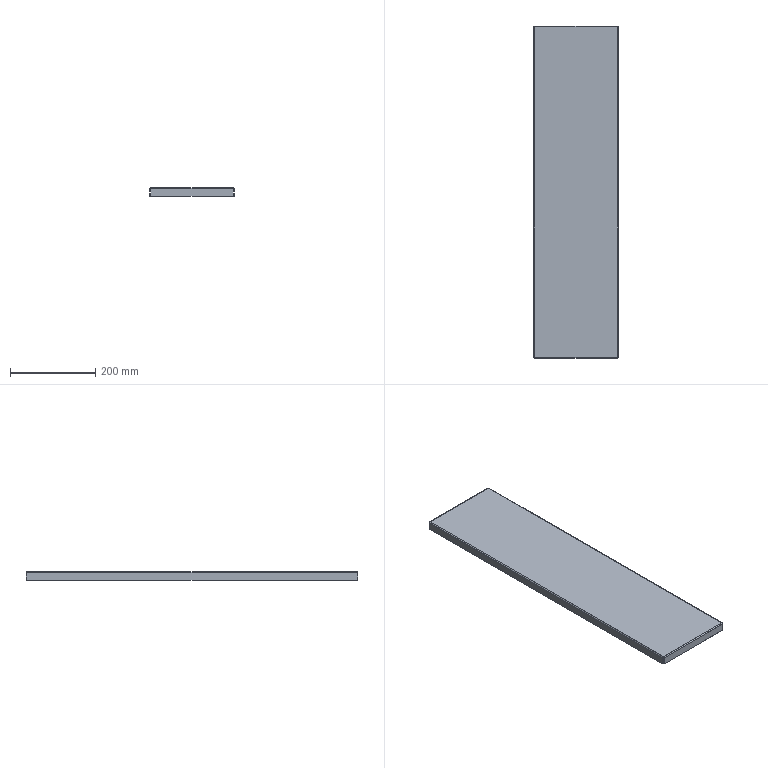Part | STEP file | X77-03019 | 1 solid | 38 faces | box 198 x 778 x 20 mm | volume 282863 mm3 | plane 22 | spline 8 | cylinder 8 | commonest cylinder face diameters 1.473 x4 4.473 x4